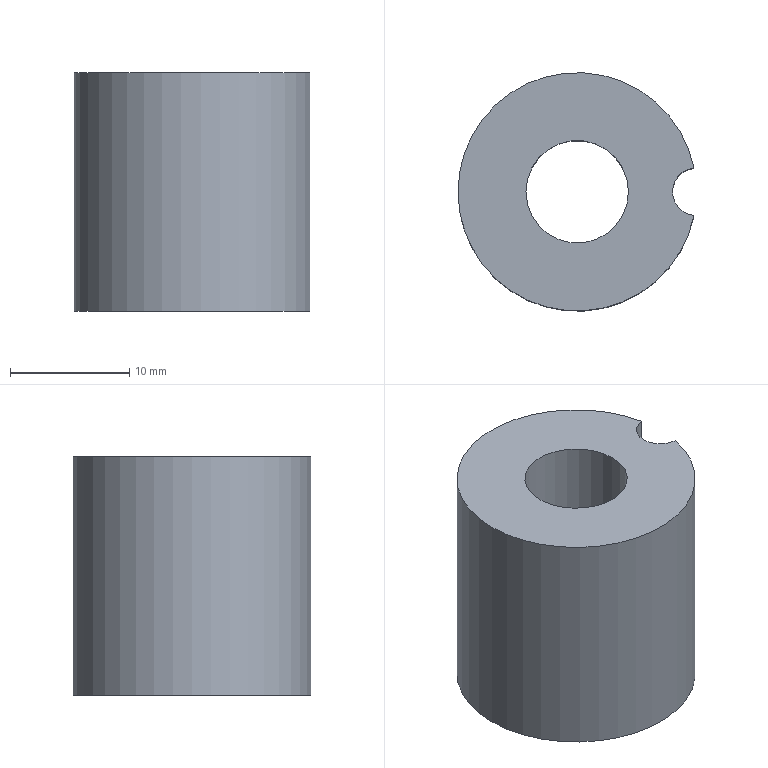Part | NX | features solid 2 | 1 solid | 7 faces | box 19.8 x 20 x 20 mm | volume 4202 mm3 | cylinder 4 | plane 3 | commonest cylinder face diameters 4 x1 8.6 x1 12.6 x1 20 x1
STEP:
#1=CARTESIAN_POINT('',(-1152.11,-325.685,77.));
#2=VERTEX_POINT('',#1);
#3=CARTESIAN_POINT('',(-1152.11,-325.685,97.));
#4=VERTEX_POINT('',#3);
#5=CARTESIAN_POINT('',(-1152.11,-325.685,87.));
#6=DIRECTION('',(0.,0.,1.));
#7=VECTOR('',#6,1000.);
#8=LINE('',#5,#7);
#9=EDGE_CURVE('',#2,#4,#8,.T.);
#10=ORIENTED_EDGE('',*,*,#9,.F.);
#11=CARTESIAN_POINT('',(-1152.11,-329.665,77.));
#12=VERTEX_POINT('',#11);
#13=CARTESIAN_POINT('',(-1161.91,-327.675,77.));
#14=DIRECTION('',(0.,0.,1.));
#15=DIRECTION('',(1.,0.,0.));
#16=AXIS2_PLACEMENT_3D('',#13,#14,#15);
#17=CIRCLE('',#16,10.);
#18=EDGE_CURVE('',#2,#12,#17,.T.);
#19=ORIENTED_EDGE('',*,*,#18,.T.);
#20=CARTESIAN_POINT('',(-1152.11,-329.665,97.));
#21=VERTEX_POINT('',#20);
#22=CARTESIAN_POINT('',(-1152.11,-329.665,87.));
#23=DIRECTION('',(0.,0.,1.));
#24=VECTOR('',#23,1000.);
#25=LINE('',#22,#24);
#26=EDGE_CURVE('',#21,#12,#25,.F.);
#27=ORIENTED_EDGE('',*,*,#26,.F.);
#28=CARTESIAN_POINT('',(-1161.91,-327.675,97.));
#29=DIRECTION('',(0.,0.,1.));
#30=DIRECTION('',(1.,0.,0.));
#31=AXIS2_PLACEMENT_3D('',#28,#29,#30);
#32=CIRCLE('',#31,10.);
#33=EDGE_CURVE('',#4,#21,#32,.T.);
#34=ORIENTED_EDGE('',*,*,#33,.F.);
#35=EDGE_LOOP('',(#10,#19,#27,#34));
#36=FACE_BOUND('',#35,.T.);
#37=CARTESIAN_POINT('',(-1161.91,-327.675,77.));
#38=DIRECTION('',(0.,0.,1.));
#39=DIRECTION('',(1.,0.,0.));
#40=AXIS2_PLACEMENT_3D('',#37,#38,#39);
#41=CYLINDRICAL_SURFACE('',#40,10.);
#42=ADVANCED_FACE('',(#36),#41,.T.);
#43=CARTESIAN_POINT('',(-1155.61,-327.675,77.));
#44=VERTEX_POINT('',#43);
#45=CARTESIAN_POINT('',(-1161.91,-327.675,77.));
#46=DIRECTION('',(0.,0.,1.));
#47=DIRECTION('',(1.,0.,0.));
#48=AXIS2_PLACEMENT_3D('',#45,#46,#47);
#49=CIRCLE('',#48,6.3);
#50=EDGE_CURVE('',#44,#44,#49,.T.);
#51=ORIENTED_EDGE('',*,*,#50,.T.);
#52=EDGE_LOOP('',(#51));
#53=FACE_BOUND('',#52,.T.);
#54=ORIENTED_EDGE('',*,*,#18,.F.);
#55=CARTESIAN_POINT('',(-1151.91,-327.675,77.));
#56=DIRECTION('',(0.,0.,1.));
#57=DIRECTION('',(1.,0.,0.));
#58=AXIS2_PLACEMENT_3D('',#55,#56,#57);
#59=CIRCLE('',#58,2.);
#60=EDGE_CURVE('',#2,#12,#59,.T.);
#61=ORIENTED_EDGE('',*,*,#60,.T.);
#62=EDGE_LOOP('',(#54,#61));
#63=FACE_BOUND('',#62,.T.);
#64=CARTESIAN_POINT('',(-1161.91,-327.675,77.));
#65=DIRECTION('',(0.,0.,1.));
#66=DIRECTION('',(1.,0.,0.));
#67=AXIS2_PLACEMENT_3D('',#64,#65,#66);
#68=PLANE('',#67);
#69=ADVANCED_FACE('',(#53,#63),#68,.F.);
#70=CARTESIAN_POINT('',(-1157.61,-327.675,97.));
#71=VERTEX_POINT('',#70);
#72=CARTESIAN_POINT('',(-1161.91,-327.675,97.));
#73=DIRECTION('',(0.,0.,1.));
#74=DIRECTION('',(1.,0.,0.));
#75=AXIS2_PLACEMENT_3D('',#72,#73,#74);
#76=CIRCLE('',#75,4.3);
#77=EDGE_CURVE('',#71,#71,#76,.T.);
#78=ORIENTED_EDGE('',*,*,#77,.F.);
#79=EDGE_LOOP('',(#78));
#80=FACE_BOUND('',#79,.T.);
#81=CARTESIAN_POINT('',(-1151.91,-327.675,97.));
#82=DIRECTION('',(0.,0.,1.));
#83=DIRECTION('',(1.,0.,0.));
#84=AXIS2_PLACEMENT_3D('',#81,#82,#83);
#85=CIRCLE('',#84,2.);
#86=EDGE_CURVE('',#4,#21,#85,.T.);
#87=ORIENTED_EDGE('',*,*,#86,.F.);
#88=ORIENTED_EDGE('',*,*,#33,.T.);
#89=EDGE_LOOP('',(#87,#88));
#90=FACE_BOUND('',#89,.T.);
#91=CARTESIAN_POINT('',(-1161.91,-327.675,97.));
#92=DIRECTION('',(0.,0.,1.));
#93=DIRECTION('',(1.,0.,0.));
#94=AXIS2_PLACEMENT_3D('',#91,#92,#93);
#95=PLANE('',#94);
#96=ADVANCED_FACE('',(#80,#90),#95,.T.);
#97=ORIENTED_EDGE('',*,*,#50,.F.);
#98=EDGE_LOOP('',(#97));
#99=FACE_BOUND('',#98,.T.);
#100=CARTESIAN_POINT('',(-1155.61,-327.675,89.));
#101=VERTEX_POINT('',#100);
#102=CARTESIAN_POINT('',(-1161.91,-327.675,89.));
#103=DIRECTION('',(0.,0.,1.));
#104=DIRECTION('',(1.,0.,0.));
#105=AXIS2_PLACEMENT_3D('',#102,#103,#104);
#106=CIRCLE('',#105,6.3);
#107=EDGE_CURVE('',#101,#101,#106,.T.);
#108=ORIENTED_EDGE('',*,*,#107,.T.);
#109=EDGE_LOOP('',(#108));
#110=FACE_BOUND('',#109,.T.);
#111=CARTESIAN_POINT('',(-1161.91,-327.675,77.));
#112=DIRECTION('',(0.,0.,1.));
#113=DIRECTION('',(1.,0.,0.));
#114=AXIS2_PLACEMENT_3D('',#111,#112,#113);
#115=CYLINDRICAL_SURFACE('',#114,6.3);
#116=ADVANCED_FACE('',(#99,#110),#115,.F.);
#117=CARTESIAN_POINT('',(-1157.61,-327.675,89.));
#118=VERTEX_POINT('',#117);
#119=CARTESIAN_POINT('',(-1161.91,-327.675,89.));
#120=DIRECTION('',(0.,0.,1.));
#121=DIRECTION('',(1.,0.,0.));
#122=AXIS2_PLACEMENT_3D('',#119,#120,#121);
#123=CIRCLE('',#122,4.3);
#124=EDGE_CURVE('',#118,#118,#123,.T.);
#125=ORIENTED_EDGE('',*,*,#124,.T.);
#126=EDGE_LOOP('',(#125));
#127=FACE_BOUND('',#126,.T.);
#128=ORIENTED_EDGE('',*,*,#107,.F.);
#129=EDGE_LOOP('',(#128));
#130=FACE_BOUND('',#129,.T.);
#131=CARTESIAN_POINT('',(-1161.91,-327.675,89.));
#132=DIRECTION('',(0.,0.,1.));
#133=DIRECTION('',(1.,0.,0.));
#134=AXIS2_PLACEMENT_3D('',#131,#132,#133);
#135=PLANE('',#134);
#136=ADVANCED_FACE('',(#127,#130),#135,.F.);
#137=ORIENTED_EDGE('',*,*,#9,.T.);
#138=ORIENTED_EDGE('',*,*,#86,.T.);
#139=ORIENTED_EDGE('',*,*,#26,.T.);
#140=ORIENTED_EDGE('',*,*,#60,.F.);
#141=EDGE_LOOP('',(#137,#138,#139,#140));
#142=FACE_BOUND('',#141,.T.);
#143=CARTESIAN_POINT('',(-1151.91,-327.675,77.));
#144=DIRECTION('',(0.,0.,1.));
#145=DIRECTION('',(1.,0.,0.));
#146=AXIS2_PLACEMENT_3D('',#143,#144,#145);
#147=CYLINDRICAL_SURFACE('',#146,2.);
#148=ADVANCED_FACE('',(#142),#147,.F.);
#149=ORIENTED_EDGE('',*,*,#77,.T.);
#150=EDGE_LOOP('',(#149));
#151=FACE_BOUND('',#150,.T.);
#152=ORIENTED_EDGE('',*,*,#124,.F.);
#153=EDGE_LOOP('',(#152));
#154=FACE_BOUND('',#153,.T.);
#155=CARTESIAN_POINT('',(-1161.91,-327.675,77.));
#156=DIRECTION('',(0.,0.,1.));
#157=DIRECTION('',(1.,0.,0.));
#158=AXIS2_PLACEMENT_3D('',#155,#156,#157);
#159=CYLINDRICAL_SURFACE('',#158,4.3);
#160=ADVANCED_FACE('',(#151,#154),#159,.F.);
#161=CLOSED_SHELL('',(#42,#69,#96,#116,#136,#148,#160));
#162=MANIFOLD_SOLID_BREP('',#161);
#163=(LENGTH_UNIT()NAMED_UNIT(*)SI_UNIT(.MILLI.,.METRE.));
#164=UNCERTAINTY_MEASURE_WITH_UNIT(LENGTH_MEASURE(0.00001),#163,'','');
#165=(NAMED_UNIT(*)PLANE_ANGLE_UNIT()SI_UNIT($,.RADIAN.));
#166=(NAMED_UNIT(*)SI_UNIT($,.STERADIAN.)SOLID_ANGLE_UNIT());
#167=(GEOMETRIC_REPRESENTATION_CONTEXT(3)GLOBAL_UNCERTAINTY_ASSIGNED_CONTEXT((#164))GLOBAL_UNIT_ASSIGNED_CONTEXT((#163,#165,#166))REPRESENTATION_CONTEXT('',''));
#168=ADVANCED_BREP_SHAPE_REPRESENTATION('',(#162),#167);